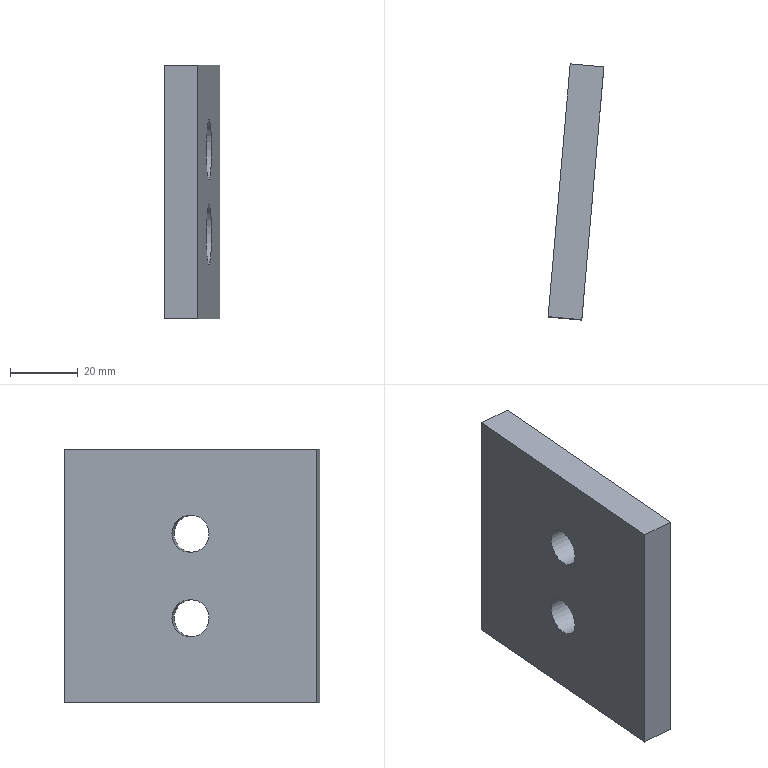Part | NX | features solid 2 | 1 solid | 12 faces | box 16.499 x 75.586 x 75 mm | volume 53488 mm3 | plane 8 | cylinder 4 | commonest cylinder face diameters 11 x2 18 x2
STEP:
#1=CARTESIAN_POINT('',(445.482,66.426,-40.626));
#2=VERTEX_POINT('',#1);
#3=CARTESIAN_POINT('',(455.444,65.555,-40.626));
#4=VERTEX_POINT('',#3);
#5=CARTESIAN_POINT('',(450.463,65.991,-40.626));
#6=DIRECTION('',(-0.9962,0.08716,0.));
#7=VECTOR('',#6,1000.);
#8=LINE('',#5,#7);
#9=EDGE_CURVE('',#2,#4,#8,.F.);
#10=ORIENTED_EDGE('',*,*,#9,.F.);
#11=CARTESIAN_POINT('',(445.482,66.426,34.374));
#12=VERTEX_POINT('',#11);
#13=CARTESIAN_POINT('',(445.482,66.426,-43.126));
#14=DIRECTION('',(0.,0.,1.));
#15=VECTOR('',#14,1000.);
#16=LINE('',#13,#15);
#17=EDGE_CURVE('',#2,#12,#16,.T.);
#18=ORIENTED_EDGE('',*,*,#17,.T.);
#19=CARTESIAN_POINT('',(455.444,65.555,34.374));
#20=VERTEX_POINT('',#19);
#21=CARTESIAN_POINT('',(450.463,65.991,34.374));
#22=DIRECTION('',(0.9962,-0.08716,0.));
#23=VECTOR('',#22,1000.);
#24=LINE('',#21,#23);
#25=EDGE_CURVE('',#12,#20,#24,.T.);
#26=ORIENTED_EDGE('',*,*,#25,.T.);
#27=CARTESIAN_POINT('',(455.444,65.555,-43.126));
#28=DIRECTION('',(0.,0.,1.));
#29=VECTOR('',#28,1000.);
#30=LINE('',#27,#29);
#31=EDGE_CURVE('',#4,#20,#30,.T.);
#32=ORIENTED_EDGE('',*,*,#31,.F.);
#33=EDGE_LOOP('',(#10,#18,#26,#32));
#34=FACE_BOUND('',#33,.T.);
#35=CARTESIAN_POINT('',(450.463,65.991,-43.126));
#36=DIRECTION('',(0.08716,0.9962,0.));
#37=DIRECTION('',(0.,0.,1.));
#38=AXIS2_PLACEMENT_3D('',#35,#36,#37);
#39=PLANE('',#38);
#40=ADVANCED_FACE('',(#34),#39,.T.);
#41=ORIENTED_EDGE('',*,*,#25,.F.);
#42=CARTESIAN_POINT('',(438.946,-8.288,34.374));
#43=VERTEX_POINT('',#42);
#44=CARTESIAN_POINT('',(445.482,66.426,34.374));
#45=DIRECTION('',(-0.08716,-0.9962,0.));
#46=VECTOR('',#45,1000.);
#47=LINE('',#44,#46);
#48=EDGE_CURVE('',#12,#43,#47,.T.);
#49=ORIENTED_EDGE('',*,*,#48,.T.);
#50=CARTESIAN_POINT('',(448.908,-9.16,34.374));
#51=VERTEX_POINT('',#50);
#52=CARTESIAN_POINT('',(443.927,-8.724,34.374));
#53=DIRECTION('',(-0.9962,0.08716,0.));
#54=VECTOR('',#53,1000.);
#55=LINE('',#52,#54);
#56=EDGE_CURVE('',#43,#51,#55,.F.);
#57=ORIENTED_EDGE('',*,*,#56,.T.);
#58=CARTESIAN_POINT('',(455.444,65.555,34.374));
#59=DIRECTION('',(-0.08716,-0.9962,0.));
#60=VECTOR('',#59,1000.);
#61=LINE('',#58,#60);
#62=EDGE_CURVE('',#20,#51,#61,.T.);
#63=ORIENTED_EDGE('',*,*,#62,.F.);
#64=EDGE_LOOP('',(#41,#49,#57,#63));
#65=FACE_BOUND('',#64,.T.);
#66=CARTESIAN_POINT('',(450.463,65.991,34.374));
#67=DIRECTION('',(0.,0.,1.));
#68=DIRECTION('',(-0.08716,-0.9962,0.));
#69=AXIS2_PLACEMENT_3D('',#66,#67,#68);
#70=PLANE('',#69);
#71=ADVANCED_FACE('',(#65),#70,.T.);
#72=ORIENTED_EDGE('',*,*,#56,.F.);
#73=CARTESIAN_POINT('',(438.946,-8.288,-40.626));
#74=VERTEX_POINT('',#73);
#75=CARTESIAN_POINT('',(438.946,-8.288,-43.126));
#76=DIRECTION('',(0.,0.,-1.));
#77=VECTOR('',#76,1000.);
#78=LINE('',#75,#77);
#79=EDGE_CURVE('',#74,#43,#78,.F.);
#80=ORIENTED_EDGE('',*,*,#79,.F.);
#81=CARTESIAN_POINT('',(448.908,-9.16,-40.626));
#82=VERTEX_POINT('',#81);
#83=CARTESIAN_POINT('',(443.927,-8.724,-40.626));
#84=DIRECTION('',(0.9962,-0.08716,0.));
#85=VECTOR('',#84,1000.);
#86=LINE('',#83,#85);
#87=EDGE_CURVE('',#74,#82,#86,.T.);
#88=ORIENTED_EDGE('',*,*,#87,.T.);
#89=CARTESIAN_POINT('',(448.908,-9.16,-43.126));
#90=DIRECTION('',(0.,0.,1.));
#91=VECTOR('',#90,1000.);
#92=LINE('',#89,#91);
#93=EDGE_CURVE('',#82,#51,#92,.T.);
#94=ORIENTED_EDGE('',*,*,#93,.T.);
#95=EDGE_LOOP('',(#72,#80,#88,#94));
#96=FACE_BOUND('',#95,.T.);
#97=CARTESIAN_POINT('',(443.927,-8.724,-43.126));
#98=DIRECTION('',(0.08716,0.9962,0.));
#99=DIRECTION('',(0.,0.,1.));
#100=AXIS2_PLACEMENT_3D('',#97,#98,#99);
#101=PLANE('',#100);
#102=ADVANCED_FACE('',(#96),#101,.F.);
#103=CARTESIAN_POINT('',(452.96,37.163,-15.626));
#104=VERTEX_POINT('',#103);
#105=CARTESIAN_POINT('',(452.176,28.198,-15.626));
#106=DIRECTION('',(0.9962,-0.08716,0.));
#107=DIRECTION('',(0.08716,0.9962,0.));
#108=AXIS2_PLACEMENT_3D('',#105,#106,#107);
#109=CIRCLE('',#108,9.);
#110=EDGE_CURVE('',#104,#104,#109,.T.);
#111=ORIENTED_EDGE('',*,*,#110,.F.);
#112=EDGE_LOOP('',(#111));
#113=FACE_BOUND('',#112,.T.);
#114=CARTESIAN_POINT('',(452.96,37.163,9.374));
#115=VERTEX_POINT('',#114);
#116=CARTESIAN_POINT('',(452.176,28.198,9.374));
#117=DIRECTION('',(0.9962,-0.08716,0.));
#118=DIRECTION('',(0.08716,0.9962,0.));
#119=AXIS2_PLACEMENT_3D('',#116,#117,#118);
#120=CIRCLE('',#119,9.);
#121=EDGE_CURVE('',#115,#115,#120,.T.);
#122=ORIENTED_EDGE('',*,*,#121,.F.);
#123=EDGE_LOOP('',(#122));
#124=FACE_BOUND('',#123,.T.);
#125=ORIENTED_EDGE('',*,*,#93,.F.);
#126=CARTESIAN_POINT('',(455.444,65.555,-40.626));
#127=DIRECTION('',(0.08716,0.9962,0.));
#128=VECTOR('',#127,1000.);
#129=LINE('',#126,#128);
#130=EDGE_CURVE('',#4,#82,#129,.F.);
#131=ORIENTED_EDGE('',*,*,#130,.F.);
#132=ORIENTED_EDGE('',*,*,#31,.T.);
#133=ORIENTED_EDGE('',*,*,#62,.T.);
#134=EDGE_LOOP('',(#125,#131,#132,#133));
#135=FACE_BOUND('',#134,.T.);
#136=CARTESIAN_POINT('',(455.444,65.555,-43.126));
#137=DIRECTION('',(0.9962,-0.08716,0.));
#138=DIRECTION('',(0.08716,0.9962,0.));
#139=AXIS2_PLACEMENT_3D('',#136,#137,#138);
#140=PLANE('',#139);
#141=ADVANCED_FACE('',(#113,#124,#135),#140,.T.);
#142=CARTESIAN_POINT('',(445.482,66.426,-40.626));
#143=DIRECTION('',(0.08716,0.9962,0.));
#144=VECTOR('',#143,1000.);
#145=LINE('',#142,#144);
#146=EDGE_CURVE('',#2,#74,#145,.F.);
#147=ORIENTED_EDGE('',*,*,#146,.F.);
#148=ORIENTED_EDGE('',*,*,#9,.T.);
#149=ORIENTED_EDGE('',*,*,#130,.T.);
#150=ORIENTED_EDGE('',*,*,#87,.F.);
#151=EDGE_LOOP('',(#147,#148,#149,#150));
#152=FACE_BOUND('',#151,.T.);
#153=CARTESIAN_POINT('',(450.463,65.991,-40.626));
#154=DIRECTION('',(0.,0.,1.));
#155=DIRECTION('',(-0.08716,-0.9962,0.));
#156=AXIS2_PLACEMENT_3D('',#153,#154,#155);
#157=PLANE('',#156);
#158=ADVANCED_FACE('',(#152),#157,.F.);
#159=CARTESIAN_POINT('',(442.693,34.548,-15.626));
#160=VERTEX_POINT('',#159);
#161=CARTESIAN_POINT('',(442.214,29.069,-15.626));
#162=DIRECTION('',(0.9962,-0.08716,0.));
#163=DIRECTION('',(0.08716,0.9962,0.));
#164=AXIS2_PLACEMENT_3D('',#161,#162,#163);
#165=CIRCLE('',#164,5.5);
#166=EDGE_CURVE('',#160,#160,#165,.T.);
#167=ORIENTED_EDGE('',*,*,#166,.T.);
#168=EDGE_LOOP('',(#167));
#169=FACE_BOUND('',#168,.T.);
#170=CARTESIAN_POINT('',(442.693,34.548,9.374));
#171=VERTEX_POINT('',#170);
#172=CARTESIAN_POINT('',(442.214,29.069,9.374));
#173=DIRECTION('',(0.9962,-0.08716,0.));
#174=DIRECTION('',(0.08716,0.9962,0.));
#175=AXIS2_PLACEMENT_3D('',#172,#173,#174);
#176=CIRCLE('',#175,5.5);
#177=EDGE_CURVE('',#171,#171,#176,.T.);
#178=ORIENTED_EDGE('',*,*,#177,.T.);
#179=EDGE_LOOP('',(#178));
#180=FACE_BOUND('',#179,.T.);
#181=ORIENTED_EDGE('',*,*,#79,.T.);
#182=ORIENTED_EDGE('',*,*,#48,.F.);
#183=ORIENTED_EDGE('',*,*,#17,.F.);
#184=ORIENTED_EDGE('',*,*,#146,.T.);
#185=EDGE_LOOP('',(#181,#182,#183,#184));
#186=FACE_BOUND('',#185,.T.);
#187=CARTESIAN_POINT('',(445.482,66.426,-43.126));
#188=DIRECTION('',(0.9962,-0.08716,0.));
#189=DIRECTION('',(0.08716,0.9962,0.));
#190=AXIS2_PLACEMENT_3D('',#187,#188,#189);
#191=PLANE('',#190);
#192=ADVANCED_FACE('',(#169,#180,#186),#191,.F.);
#193=CARTESIAN_POINT('',(449.007,22.954,9.374));
#194=VERTEX_POINT('',#193);
#195=CARTESIAN_POINT('',(449.486,28.433,9.374));
#196=DIRECTION('',(-0.9962,0.08716,0.));
#197=DIRECTION('',(-0.08716,-0.9962,0.));
#198=AXIS2_PLACEMENT_3D('',#195,#196,#197);
#199=CIRCLE('',#198,5.5);
#200=EDGE_CURVE('',#194,#194,#199,.F.);
#201=ORIENTED_EDGE('',*,*,#200,.T.);
#202=EDGE_LOOP('',(#201));
#203=FACE_BOUND('',#202,.T.);
#204=ORIENTED_EDGE('',*,*,#177,.F.);
#205=EDGE_LOOP('',(#204));
#206=FACE_BOUND('',#205,.T.);
#207=CARTESIAN_POINT('',(434.942,29.705,9.374));
#208=DIRECTION('',(0.9962,-0.08716,0.));
#209=DIRECTION('',(0.08716,0.9962,0.));
#210=AXIS2_PLACEMENT_3D('',#207,#208,#209);
#211=CYLINDRICAL_SURFACE('',#210,5.5);
#212=ADVANCED_FACE('',(#203,#206),#211,.F.);
#213=ORIENTED_EDGE('',*,*,#200,.F.);
#214=EDGE_LOOP('',(#213));
#215=FACE_BOUND('',#214,.T.);
#216=CARTESIAN_POINT('',(450.271,37.399,9.374));
#217=VERTEX_POINT('',#216);
#218=CARTESIAN_POINT('',(449.486,28.433,9.374));
#219=DIRECTION('',(0.9962,-0.08716,0.));
#220=DIRECTION('',(0.08716,0.9962,0.));
#221=AXIS2_PLACEMENT_3D('',#218,#219,#220);
#222=CIRCLE('',#221,9.);
#223=EDGE_CURVE('',#217,#217,#222,.T.);
#224=ORIENTED_EDGE('',*,*,#223,.T.);
#225=EDGE_LOOP('',(#224));
#226=FACE_BOUND('',#225,.T.);
#227=CARTESIAN_POINT('',(449.486,28.433,9.374));
#228=DIRECTION('',(-0.9962,0.08716,0.));
#229=DIRECTION('',(-0.08716,-0.9962,0.));
#230=AXIS2_PLACEMENT_3D('',#227,#228,#229);
#231=PLANE('',#230);
#232=ADVANCED_FACE('',(#215,#226),#231,.F.);
#233=ORIENTED_EDGE('',*,*,#121,.T.);
#234=EDGE_LOOP('',(#233));
#235=FACE_BOUND('',#234,.T.);
#236=ORIENTED_EDGE('',*,*,#223,.F.);
#237=EDGE_LOOP('',(#236));
#238=FACE_BOUND('',#237,.T.);
#239=CARTESIAN_POINT('',(449.486,28.433,9.374));
#240=DIRECTION('',(0.9962,-0.08716,0.));
#241=DIRECTION('',(0.08716,0.9962,0.));
#242=AXIS2_PLACEMENT_3D('',#239,#240,#241);
#243=CYLINDRICAL_SURFACE('',#242,9.);
#244=ADVANCED_FACE('',(#235,#238),#243,.F.);
#245=CARTESIAN_POINT('',(449.007,22.954,-15.626));
#246=VERTEX_POINT('',#245);
#247=CARTESIAN_POINT('',(449.486,28.433,-15.626));
#248=DIRECTION('',(-0.9962,0.08716,0.));
#249=DIRECTION('',(-0.08716,-0.9962,0.));
#250=AXIS2_PLACEMENT_3D('',#247,#248,#249);
#251=CIRCLE('',#250,5.5);
#252=EDGE_CURVE('',#246,#246,#251,.F.);
#253=ORIENTED_EDGE('',*,*,#252,.T.);
#254=EDGE_LOOP('',(#253));
#255=FACE_BOUND('',#254,.T.);
#256=ORIENTED_EDGE('',*,*,#166,.F.);
#257=EDGE_LOOP('',(#256));
#258=FACE_BOUND('',#257,.T.);
#259=CARTESIAN_POINT('',(434.942,29.705,-15.626));
#260=DIRECTION('',(0.9962,-0.08716,0.));
#261=DIRECTION('',(0.08716,0.9962,0.));
#262=AXIS2_PLACEMENT_3D('',#259,#260,#261);
#263=CYLINDRICAL_SURFACE('',#262,5.5);
#264=ADVANCED_FACE('',(#255,#258),#263,.F.);
#265=ORIENTED_EDGE('',*,*,#252,.F.);
#266=EDGE_LOOP('',(#265));
#267=FACE_BOUND('',#266,.T.);
#268=CARTESIAN_POINT('',(450.271,37.399,-15.626));
#269=VERTEX_POINT('',#268);
#270=CARTESIAN_POINT('',(449.486,28.433,-15.626));
#271=DIRECTION('',(0.9962,-0.08716,0.));
#272=DIRECTION('',(0.08716,0.9962,0.));
#273=AXIS2_PLACEMENT_3D('',#270,#271,#272);
#274=CIRCLE('',#273,9.);
#275=EDGE_CURVE('',#269,#269,#274,.T.);
#276=ORIENTED_EDGE('',*,*,#275,.T.);
#277=EDGE_LOOP('',(#276));
#278=FACE_BOUND('',#277,.T.);
#279=CARTESIAN_POINT('',(449.486,28.433,-15.626));
#280=DIRECTION('',(-0.9962,0.08716,0.));
#281=DIRECTION('',(-0.08716,-0.9962,0.));
#282=AXIS2_PLACEMENT_3D('',#279,#280,#281);
#283=PLANE('',#282);
#284=ADVANCED_FACE('',(#267,#278),#283,.F.);
#285=ORIENTED_EDGE('',*,*,#110,.T.);
#286=EDGE_LOOP('',(#285));
#287=FACE_BOUND('',#286,.T.);
#288=ORIENTED_EDGE('',*,*,#275,.F.);
#289=EDGE_LOOP('',(#288));
#290=FACE_BOUND('',#289,.T.);
#291=CARTESIAN_POINT('',(449.486,28.433,-15.626));
#292=DIRECTION('',(0.9962,-0.08716,0.));
#293=DIRECTION('',(0.08716,0.9962,0.));
#294=AXIS2_PLACEMENT_3D('',#291,#292,#293);
#295=CYLINDRICAL_SURFACE('',#294,9.);
#296=ADVANCED_FACE('',(#287,#290),#295,.F.);
#297=CLOSED_SHELL('',(#40,#71,#102,#141,#158,#192,#212,#232,#244,#264,#284,#296));
#298=MANIFOLD_SOLID_BREP('',#297);
#299=(LENGTH_UNIT()NAMED_UNIT(*)SI_UNIT(.MILLI.,.METRE.));
#300=UNCERTAINTY_MEASURE_WITH_UNIT(LENGTH_MEASURE(0.00001),#299,'','');
#301=(NAMED_UNIT(*)PLANE_ANGLE_UNIT()SI_UNIT($,.RADIAN.));
#302=(NAMED_UNIT(*)SI_UNIT($,.STERADIAN.)SOLID_ANGLE_UNIT());
#303=(GEOMETRIC_REPRESENTATION_CONTEXT(3)GLOBAL_UNCERTAINTY_ASSIGNED_CONTEXT((#300))GLOBAL_UNIT_ASSIGNED_CONTEXT((#299,#301,#302))REPRESENTATION_CONTEXT('',''));
#304=ADVANCED_BREP_SHAPE_REPRESENTATION('',(#298),#303);